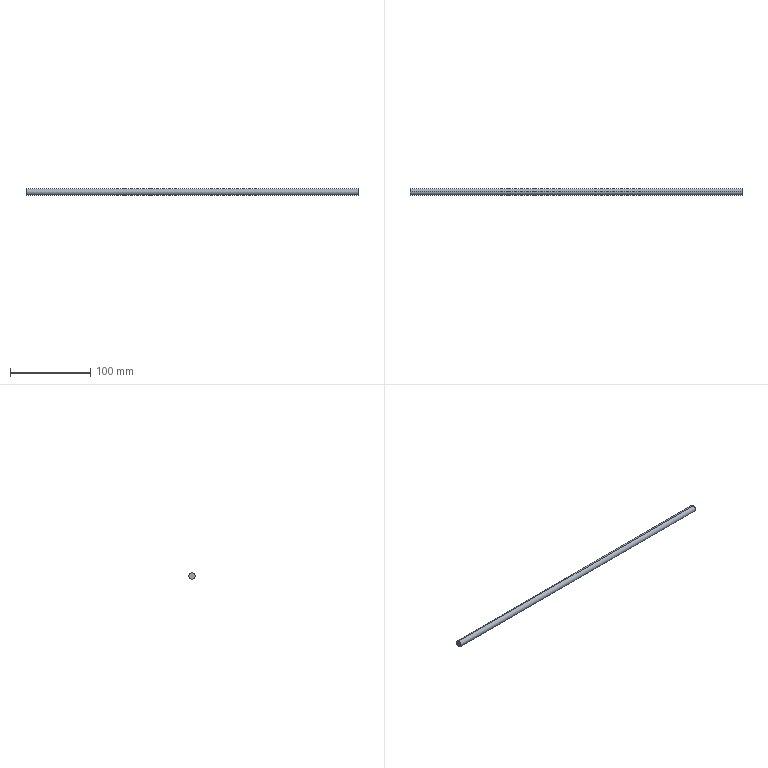Part | STEP file | Tie bar | 1 solid | 4 faces | box 415 x 8 x 8 mm | volume 20860 mm3 | cylinder 2 | plane 2 | commonest cylinder face diameters 8 x2
STEP:
#1=CARTESIAN_POINT('',(0.,0.,0.));
#2=DIRECTION('',(0.,0.,1.));
#3=DIRECTION('',(1.,0.,0.));
#4=AXIS2_PLACEMENT_3D('',#1,#2,#3);
#5=CARTESIAN_POINT('',(207.5,0.,-4.));
#6=VERTEX_POINT('',#5);
#7=CARTESIAN_POINT('',(207.5,0.,4.));
#8=VERTEX_POINT('',#7);
#9=CARTESIAN_POINT('',(207.5,0.,0.));
#10=DIRECTION('',(1.,0.,0.));
#11=DIRECTION('',(0.,0.,-1.));
#12=AXIS2_PLACEMENT_3D('',#9,#10,#11);
#13=CIRCLE('',#12,4.);
#14=CARTESIAN_POINT('',(207.5,0.,0.));
#15=DIRECTION('',(-1.,0.,0.));
#16=DIRECTION('',(0.,0.,1.));
#17=AXIS2_PLACEMENT_3D('',#14,#15,#16);
#18=CYLINDRICAL_SURFACE('',#17,4.);
#19=CARTESIAN_POINT('',(3.142,0.));
#20=DIRECTION('',(-1.,0.));
#21=VECTOR('',#20,1.);
#22=LINE('',#19,#21);
#23=(GEOMETRIC_REPRESENTATION_CONTEXT(2)PARAMETRIC_REPRESENTATION_CONTEXT()REPRESENTATION_CONTEXT('',''));
#24=DEFINITIONAL_REPRESENTATION('',(#22),#23);
#25=PCURVE('',#18,#24);
#26=CARTESIAN_POINT('',(207.5,0.,0.));
#27=DIRECTION('',(1.,0.,0.));
#28=DIRECTION('',(0.,0.,-1.));
#29=AXIS2_PLACEMENT_3D('',#26,#27,#28);
#30=PLANE('',#29);
#31=CARTESIAN_POINT('',(0.,0.));
#32=DIRECTION('',(1.,0.));
#33=AXIS2_PLACEMENT_2D('',#31,#32);
#34=CIRCLE('',#33,4.);
#35=(GEOMETRIC_REPRESENTATION_CONTEXT(2)PARAMETRIC_REPRESENTATION_CONTEXT()REPRESENTATION_CONTEXT('',''));
#36=DEFINITIONAL_REPRESENTATION('',(#34),#35);
#37=PCURVE('',#30,#36);
#38=SURFACE_CURVE('',#13,(#25,#37),.PCURVE_S1.);
#39=EDGE_CURVE('',#6,#8,#38,.T.);
#40=ORIENTED_EDGE('',*,*,#39,.F.);
#41=CARTESIAN_POINT('',(-207.5,0.,-4.));
#42=VERTEX_POINT('',#41);
#43=CARTESIAN_POINT('',(207.5,0.,-4.));
#44=DIRECTION('',(-1.,0.,0.));
#45=VECTOR('',#44,1.);
#46=LINE('',#43,#45);
#47=CARTESIAN_POINT('',(3.142,0.));
#48=DIRECTION('',(0.,1.));
#49=VECTOR('',#48,1.);
#50=LINE('',#47,#49);
#51=(GEOMETRIC_REPRESENTATION_CONTEXT(2)PARAMETRIC_REPRESENTATION_CONTEXT()REPRESENTATION_CONTEXT('',''));
#52=DEFINITIONAL_REPRESENTATION('',(#50),#51);
#53=PCURVE('',#18,#52);
#54=CARTESIAN_POINT('',(207.5,0.,0.));
#55=DIRECTION('',(-1.,0.,0.));
#56=DIRECTION('',(0.,0.,1.));
#57=AXIS2_PLACEMENT_3D('',#54,#55,#56);
#58=CYLINDRICAL_SURFACE('',#57,4.);
#59=CARTESIAN_POINT('',(3.142,0.));
#60=DIRECTION('',(0.,1.));
#61=VECTOR('',#60,1.);
#62=LINE('',#59,#61);
#63=(GEOMETRIC_REPRESENTATION_CONTEXT(2)PARAMETRIC_REPRESENTATION_CONTEXT()REPRESENTATION_CONTEXT('',''));
#64=DEFINITIONAL_REPRESENTATION('',(#62),#63);
#65=PCURVE('',#58,#64);
#66=SURFACE_CURVE('',#46,(#53,#65),.PCURVE_S1.);
#67=EDGE_CURVE('',#6,#42,#66,.T.);
#68=ORIENTED_EDGE('',*,*,#67,.T.);
#69=CARTESIAN_POINT('',(-207.5,0.,4.));
#70=VERTEX_POINT('',#69);
#71=CARTESIAN_POINT('',(-207.5,0.,0.));
#72=DIRECTION('',(1.,0.,0.));
#73=DIRECTION('',(0.,0.,-1.));
#74=AXIS2_PLACEMENT_3D('',#71,#72,#73);
#75=CIRCLE('',#74,4.);
#76=CARTESIAN_POINT('',(3.142,415.));
#77=DIRECTION('',(-1.,0.));
#78=VECTOR('',#77,1.);
#79=LINE('',#76,#78);
#80=(GEOMETRIC_REPRESENTATION_CONTEXT(2)PARAMETRIC_REPRESENTATION_CONTEXT()REPRESENTATION_CONTEXT('',''));
#81=DEFINITIONAL_REPRESENTATION('',(#79),#80);
#82=PCURVE('',#18,#81);
#83=CARTESIAN_POINT('',(-207.5,0.,0.));
#84=DIRECTION('',(1.,0.,0.));
#85=DIRECTION('',(0.,0.,-1.));
#86=AXIS2_PLACEMENT_3D('',#83,#84,#85);
#87=PLANE('',#86);
#88=CARTESIAN_POINT('',(0.,0.));
#89=DIRECTION('',(1.,0.));
#90=AXIS2_PLACEMENT_2D('',#88,#89);
#91=CIRCLE('',#90,4.);
#92=(GEOMETRIC_REPRESENTATION_CONTEXT(2)PARAMETRIC_REPRESENTATION_CONTEXT()REPRESENTATION_CONTEXT('',''));
#93=DEFINITIONAL_REPRESENTATION('',(#91),#92);
#94=PCURVE('',#87,#93);
#95=SURFACE_CURVE('',#75,(#82,#94),.PCURVE_S1.);
#96=EDGE_CURVE('',#42,#70,#95,.T.);
#97=ORIENTED_EDGE('',*,*,#96,.T.);
#98=CARTESIAN_POINT('',(207.5,0.,4.));
#99=DIRECTION('',(-1.,0.,0.));
#100=VECTOR('',#99,1.);
#101=LINE('',#98,#100);
#102=CARTESIAN_POINT('',(0.,0.));
#103=DIRECTION('',(0.,1.));
#104=VECTOR('',#103,1.);
#105=LINE('',#102,#104);
#106=(GEOMETRIC_REPRESENTATION_CONTEXT(2)PARAMETRIC_REPRESENTATION_CONTEXT()REPRESENTATION_CONTEXT('',''));
#107=DEFINITIONAL_REPRESENTATION('',(#105),#106);
#108=PCURVE('',#18,#107);
#109=CARTESIAN_POINT('',(6.283,0.));
#110=DIRECTION('',(0.,1.));
#111=VECTOR('',#110,1.);
#112=LINE('',#109,#111);
#113=(GEOMETRIC_REPRESENTATION_CONTEXT(2)PARAMETRIC_REPRESENTATION_CONTEXT()REPRESENTATION_CONTEXT('',''));
#114=DEFINITIONAL_REPRESENTATION('',(#112),#113);
#115=PCURVE('',#58,#114);
#116=SURFACE_CURVE('',#101,(#108,#115),.PCURVE_S1.);
#117=EDGE_CURVE('',#8,#70,#116,.T.);
#118=ORIENTED_EDGE('',*,*,#117,.F.);
#119=EDGE_LOOP('',(#40,#68,#97,#118));
#120=FACE_BOUND('',#119,.T.);
#121=ADVANCED_FACE('',(#120),#18,.T.);
#122=ORIENTED_EDGE('',*,*,#67,.F.);
#123=CARTESIAN_POINT('',(207.5,0.,0.));
#124=DIRECTION('',(1.,0.,0.));
#125=DIRECTION('',(0.,0.,-1.));
#126=AXIS2_PLACEMENT_3D('',#123,#124,#125);
#127=CIRCLE('',#126,4.);
#128=CARTESIAN_POINT('',(9.425,0.));
#129=DIRECTION('',(-1.,0.));
#130=VECTOR('',#129,1.);
#131=LINE('',#128,#130);
#132=(GEOMETRIC_REPRESENTATION_CONTEXT(2)PARAMETRIC_REPRESENTATION_CONTEXT()REPRESENTATION_CONTEXT('',''));
#133=DEFINITIONAL_REPRESENTATION('',(#131),#132);
#134=PCURVE('',#58,#133);
#135=CARTESIAN_POINT('',(0.,0.));
#136=DIRECTION('',(1.,0.));
#137=AXIS2_PLACEMENT_2D('',#135,#136);
#138=CIRCLE('',#137,4.);
#139=(GEOMETRIC_REPRESENTATION_CONTEXT(2)PARAMETRIC_REPRESENTATION_CONTEXT()REPRESENTATION_CONTEXT('',''));
#140=DEFINITIONAL_REPRESENTATION('',(#138),#139);
#141=PCURVE('',#30,#140);
#142=SURFACE_CURVE('',#127,(#134,#141),.PCURVE_S1.);
#143=EDGE_CURVE('',#8,#6,#142,.T.);
#144=ORIENTED_EDGE('',*,*,#143,.F.);
#145=ORIENTED_EDGE('',*,*,#117,.T.);
#146=CARTESIAN_POINT('',(-207.5,0.,0.));
#147=DIRECTION('',(1.,0.,0.));
#148=DIRECTION('',(0.,0.,-1.));
#149=AXIS2_PLACEMENT_3D('',#146,#147,#148);
#150=CIRCLE('',#149,4.);
#151=CARTESIAN_POINT('',(9.425,415.));
#152=DIRECTION('',(-1.,0.));
#153=VECTOR('',#152,1.);
#154=LINE('',#151,#153);
#155=(GEOMETRIC_REPRESENTATION_CONTEXT(2)PARAMETRIC_REPRESENTATION_CONTEXT()REPRESENTATION_CONTEXT('',''));
#156=DEFINITIONAL_REPRESENTATION('',(#154),#155);
#157=PCURVE('',#58,#156);
#158=CARTESIAN_POINT('',(0.,0.));
#159=DIRECTION('',(1.,0.));
#160=AXIS2_PLACEMENT_2D('',#158,#159);
#161=CIRCLE('',#160,4.);
#162=(GEOMETRIC_REPRESENTATION_CONTEXT(2)PARAMETRIC_REPRESENTATION_CONTEXT()REPRESENTATION_CONTEXT('',''));
#163=DEFINITIONAL_REPRESENTATION('',(#161),#162);
#164=PCURVE('',#87,#163);
#165=SURFACE_CURVE('',#150,(#157,#164),.PCURVE_S1.);
#166=EDGE_CURVE('',#70,#42,#165,.T.);
#167=ORIENTED_EDGE('',*,*,#166,.T.);
#168=EDGE_LOOP('',(#122,#144,#145,#167));
#169=FACE_BOUND('',#168,.T.);
#170=ADVANCED_FACE('',(#169),#58,.T.);
#171=ORIENTED_EDGE('',*,*,#143,.T.);
#172=ORIENTED_EDGE('',*,*,#39,.T.);
#173=EDGE_LOOP('',(#171,#172));
#174=FACE_BOUND('',#173,.T.);
#175=ADVANCED_FACE('',(#174),#30,.T.);
#176=ORIENTED_EDGE('',*,*,#166,.F.);
#177=ORIENTED_EDGE('',*,*,#96,.F.);
#178=EDGE_LOOP('',(#176,#177));
#179=FACE_BOUND('',#178,.T.);
#180=ADVANCED_FACE('',(#179),#87,.F.);
#181=CLOSED_SHELL('',(#121,#170,#175,#180));
#182=MANIFOLD_SOLID_BREP('',#181);
#183=(LENGTH_UNIT()NAMED_UNIT(*)SI_UNIT(.MILLI.,.METRE.));
#184=UNCERTAINTY_MEASURE_WITH_UNIT(LENGTH_MEASURE(0.0000001),#183,'','');
#185=(NAMED_UNIT(*)PLANE_ANGLE_UNIT()SI_UNIT($,.RADIAN.));
#186=(NAMED_UNIT(*)SI_UNIT($,.STERADIAN.)SOLID_ANGLE_UNIT());
#187=(GEOMETRIC_REPRESENTATION_CONTEXT(3)GLOBAL_UNCERTAINTY_ASSIGNED_CONTEXT((#184))GLOBAL_UNIT_ASSIGNED_CONTEXT((#183,#185,#186))REPRESENTATION_CONTEXT('',''));
#188=ADVANCED_BREP_SHAPE_REPRESENTATION('',(#4,#182),#187);